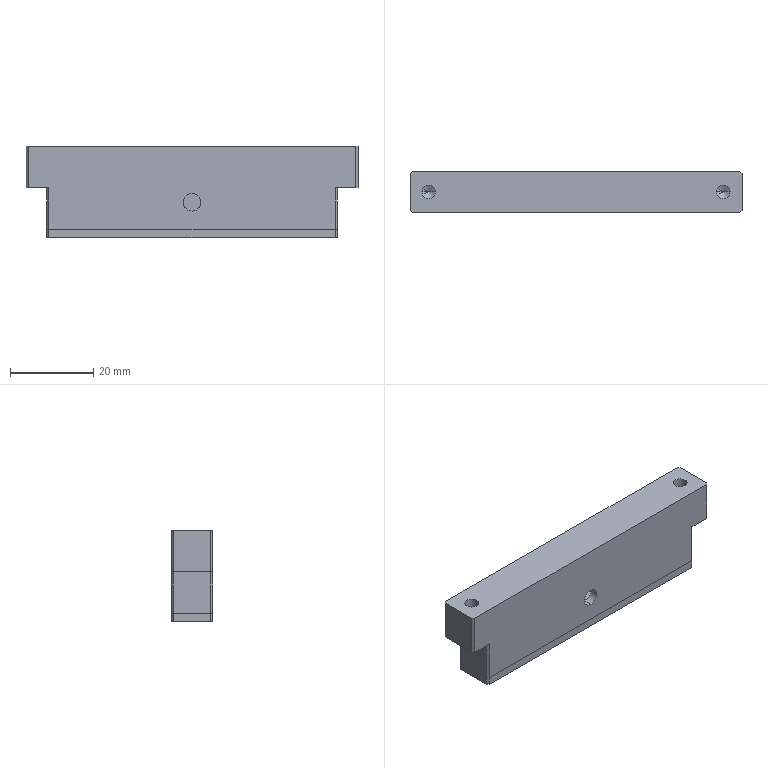Part | SolidWorks | features ICE 6, Chamfer 2, HoleWzd 2, Extrusion 1, LPattern 1 | 3 solids | 231 faces | box 80 x 10 x 22 mm | volume 14660 mm3 | cylinder 182 | plane 45 | cone 4 | commonest cylinder face diameters 1 x176 3.3 x4 4.2 x2